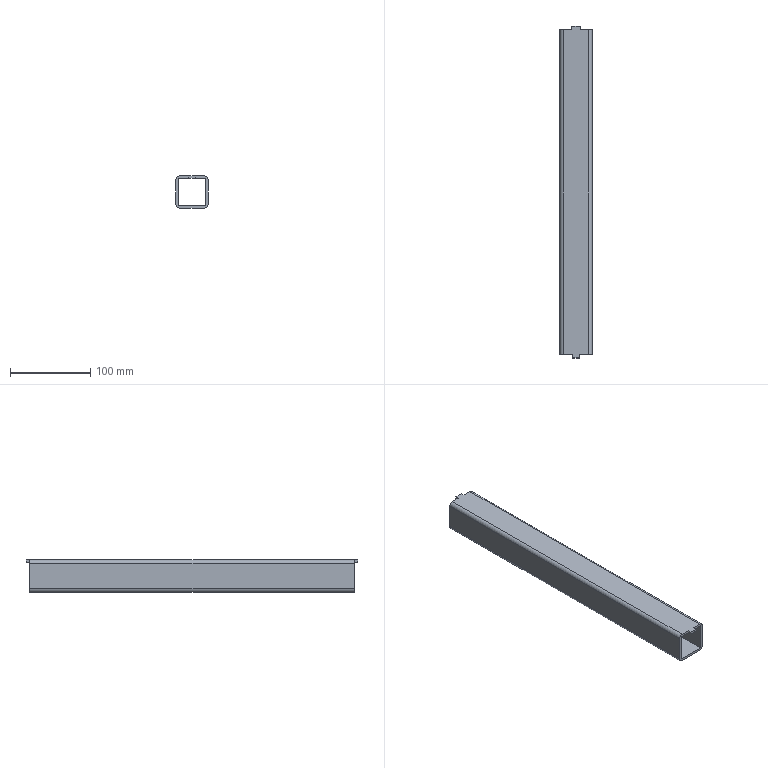Part | 1 solid | 20 faces | box 40 x 414 x 40 mm | volume 173023 mm3 | plane 16 | cylinder 4 | commonest cylinder face diameters 9 x4
STEP:
#1=CARTESIAN_POINT('',(-268.,85.,604.5));
#2=VERTEX_POINT('',#1);
#3=CARTESIAN_POINT('',(-268.,85.,635.5));
#4=VERTEX_POINT('',#3);
#5=CARTESIAN_POINT('',(-268.,85.,600.));
#6=DIRECTION('',(0.,0.,1.));
#7=VECTOR('',#6,1000.);
#8=LINE('',#5,#7);
#9=EDGE_CURVE('',#2,#4,#8,.T.);
#10=ORIENTED_EDGE('',*,*,#9,.F.);
#11=CARTESIAN_POINT('',(-268.,490.,604.5));
#12=VERTEX_POINT('',#11);
#13=CARTESIAN_POINT('',(-268.,490.,604.5));
#14=DIRECTION('',(0.,1.,0.));
#15=VECTOR('',#14,1000.);
#16=LINE('',#13,#15);
#17=EDGE_CURVE('',#2,#12,#16,.T.);
#18=ORIENTED_EDGE('',*,*,#17,.T.);
#19=CARTESIAN_POINT('',(-268.,490.,635.5));
#20=VERTEX_POINT('',#19);
#21=CARTESIAN_POINT('',(-268.,490.,600.));
#22=DIRECTION('',(0.,0.,1.));
#23=VECTOR('',#22,1000.);
#24=LINE('',#21,#23);
#25=EDGE_CURVE('',#12,#20,#24,.T.);
#26=ORIENTED_EDGE('',*,*,#25,.T.);
#27=CARTESIAN_POINT('',(-268.,40.,635.5));
#28=DIRECTION('',(0.,-1.,0.));
#29=VECTOR('',#28,1000.);
#30=LINE('',#27,#29);
#31=EDGE_CURVE('',#20,#4,#30,.T.);
#32=ORIENTED_EDGE('',*,*,#31,.T.);
#33=EDGE_LOOP('',(#10,#18,#26,#32));
#34=FACE_OUTER_BOUND('',#33,.T.);
#35=CARTESIAN_POINT('',(-268.,40.,600.));
#36=DIRECTION('',(1.,0.,0.));
#37=DIRECTION('',(0.,0.,-1.));
#38=AXIS2_PLACEMENT_3D('',#35,#36,#37);
#39=PLANE('',#38);
#40=ADVANCED_FACE('',(#34),#39,.T.);
#41=CARTESIAN_POINT('',(-308.,85.,604.5));
#42=VERTEX_POINT('',#41);
#43=CARTESIAN_POINT('',(-308.,85.,635.5));
#44=VERTEX_POINT('',#43);
#45=CARTESIAN_POINT('',(-308.,85.,600.));
#46=DIRECTION('',(0.,0.,1.));
#47=VECTOR('',#46,1000.);
#48=LINE('',#45,#47);
#49=EDGE_CURVE('',#42,#44,#48,.T.);
#50=ORIENTED_EDGE('',*,*,#49,.F.);
#51=CARTESIAN_POINT('',(-303.5,85.,600.));
#52=VERTEX_POINT('',#51);
#53=CARTESIAN_POINT('',(-303.5,85.,604.5));
#54=DIRECTION('',(0.,-1.,0.));
#55=DIRECTION('',(0.,0.,-1.));
#56=AXIS2_PLACEMENT_3D('',#53,#54,#55);
#57=CIRCLE('',#56,4.5);
#58=EDGE_CURVE('',#42,#52,#57,.T.);
#59=ORIENTED_EDGE('',*,*,#58,.T.);
#60=CARTESIAN_POINT('',(-272.5,85.,600.));
#61=VERTEX_POINT('',#60);
#62=CARTESIAN_POINT('',(-308.,85.,600.));
#63=DIRECTION('',(1.,0.,0.));
#64=VECTOR('',#63,1000.);
#65=LINE('',#62,#64);
#66=EDGE_CURVE('',#52,#61,#65,.T.);
#67=ORIENTED_EDGE('',*,*,#66,.T.);
#68=CARTESIAN_POINT('',(-272.5,85.,604.5));
#69=DIRECTION('',(0.,-1.,0.));
#70=DIRECTION('',(0.,0.,-1.));
#71=AXIS2_PLACEMENT_3D('',#68,#69,#70);
#72=CIRCLE('',#71,4.5);
#73=EDGE_CURVE('',#61,#2,#72,.T.);
#74=ORIENTED_EDGE('',*,*,#73,.T.);
#75=ORIENTED_EDGE('',*,*,#9,.T.);
#76=CARTESIAN_POINT('',(-272.5,85.,640.));
#77=VERTEX_POINT('',#76);
#78=CARTESIAN_POINT('',(-272.5,85.,635.5));
#79=DIRECTION('',(0.,-1.,0.));
#80=DIRECTION('',(0.,0.,-1.));
#81=AXIS2_PLACEMENT_3D('',#78,#79,#80);
#82=CIRCLE('',#81,4.5);
#83=EDGE_CURVE('',#4,#77,#82,.T.);
#84=ORIENTED_EDGE('',*,*,#83,.T.);
#85=CARTESIAN_POINT('',(-284.,85.,640.));
#86=VERTEX_POINT('',#85);
#87=CARTESIAN_POINT('',(-308.,85.,640.));
#88=DIRECTION('',(1.,0.,0.));
#89=VECTOR('',#88,1000.);
#90=LINE('',#87,#89);
#91=EDGE_CURVE('',#86,#77,#90,.T.);
#92=ORIENTED_EDGE('',*,*,#91,.F.);
#93=CARTESIAN_POINT('',(-284.,85.,637.));
#94=VERTEX_POINT('',#93);
#95=CARTESIAN_POINT('',(-284.,85.,640.));
#96=DIRECTION('',(0.,0.,1.));
#97=VECTOR('',#96,1000.);
#98=LINE('',#95,#97);
#99=EDGE_CURVE('',#94,#86,#98,.T.);
#100=ORIENTED_EDGE('',*,*,#99,.F.);
#101=CARTESIAN_POINT('',(-271.,85.,637.));
#102=VERTEX_POINT('',#101);
#103=CARTESIAN_POINT('',(-305.,85.,637.));
#104=DIRECTION('',(1.,0.,0.));
#105=VECTOR('',#104,1000.);
#106=LINE('',#103,#105);
#107=EDGE_CURVE('',#94,#102,#106,.T.);
#108=ORIENTED_EDGE('',*,*,#107,.T.);
#109=CARTESIAN_POINT('',(-271.,85.,603.));
#110=VERTEX_POINT('',#109);
#111=CARTESIAN_POINT('',(-271.,85.,637.));
#112=DIRECTION('',(0.,0.,-1.));
#113=VECTOR('',#112,1000.);
#114=LINE('',#111,#113);
#115=EDGE_CURVE('',#102,#110,#114,.T.);
#116=ORIENTED_EDGE('',*,*,#115,.T.);
#117=CARTESIAN_POINT('',(-305.,85.,603.));
#118=VERTEX_POINT('',#117);
#119=CARTESIAN_POINT('',(-271.,85.,603.));
#120=DIRECTION('',(-1.,0.,0.));
#121=VECTOR('',#120,1000.);
#122=LINE('',#119,#121);
#123=EDGE_CURVE('',#110,#118,#122,.T.);
#124=ORIENTED_EDGE('',*,*,#123,.T.);
#125=CARTESIAN_POINT('',(-305.,85.,637.));
#126=VERTEX_POINT('',#125);
#127=CARTESIAN_POINT('',(-305.,85.,603.));
#128=DIRECTION('',(0.,0.,1.));
#129=VECTOR('',#128,1000.);
#130=LINE('',#127,#129);
#131=EDGE_CURVE('',#118,#126,#130,.T.);
#132=ORIENTED_EDGE('',*,*,#131,.T.);
#133=CARTESIAN_POINT('',(-292.,85.,637.));
#134=VERTEX_POINT('',#133);
#135=CARTESIAN_POINT('',(-305.,85.,637.));
#136=DIRECTION('',(1.,0.,0.));
#137=VECTOR('',#136,1000.);
#138=LINE('',#135,#137);
#139=EDGE_CURVE('',#126,#134,#138,.T.);
#140=ORIENTED_EDGE('',*,*,#139,.T.);
#141=CARTESIAN_POINT('',(-292.,85.,640.));
#142=VERTEX_POINT('',#141);
#143=CARTESIAN_POINT('',(-292.,85.,637.));
#144=DIRECTION('',(0.,0.,-1.));
#145=VECTOR('',#144,1000.);
#146=LINE('',#143,#145);
#147=EDGE_CURVE('',#142,#134,#146,.T.);
#148=ORIENTED_EDGE('',*,*,#147,.F.);
#149=CARTESIAN_POINT('',(-303.5,85.,640.));
#150=VERTEX_POINT('',#149);
#151=CARTESIAN_POINT('',(-308.,85.,640.));
#152=DIRECTION('',(1.,0.,0.));
#153=VECTOR('',#152,1000.);
#154=LINE('',#151,#153);
#155=EDGE_CURVE('',#150,#142,#154,.T.);
#156=ORIENTED_EDGE('',*,*,#155,.F.);
#157=CARTESIAN_POINT('',(-303.5,85.,635.5));
#158=DIRECTION('',(0.,-1.,0.));
#159=DIRECTION('',(0.,0.,-1.));
#160=AXIS2_PLACEMENT_3D('',#157,#158,#159);
#161=CIRCLE('',#160,4.5);
#162=EDGE_CURVE('',#150,#44,#161,.T.);
#163=ORIENTED_EDGE('',*,*,#162,.T.);
#164=EDGE_LOOP('',(#50,#59,#67,#74,#75,#84,#92,#100,#108,#116,#124,#132,#140,#148,#156,#163));
#165=FACE_OUTER_BOUND('',#164,.T.);
#166=CARTESIAN_POINT('',(-308.,85.,600.));
#167=DIRECTION('',(0.,-1.,0.));
#168=DIRECTION('',(0.,0.,-1.));
#169=AXIS2_PLACEMENT_3D('',#166,#167,#168);
#170=PLANE('',#169);
#171=ADVANCED_FACE('',(#165),#170,.T.);
#172=CARTESIAN_POINT('',(-308.,490.,604.5));
#173=VERTEX_POINT('',#172);
#174=CARTESIAN_POINT('',(-308.,490.,635.5));
#175=VERTEX_POINT('',#174);
#176=CARTESIAN_POINT('',(-308.,490.,600.));
#177=DIRECTION('',(0.,0.,1.));
#178=VECTOR('',#177,1000.);
#179=LINE('',#176,#178);
#180=EDGE_CURVE('',#173,#175,#179,.T.);
#181=ORIENTED_EDGE('',*,*,#180,.F.);
#182=CARTESIAN_POINT('',(-308.,40.,604.5));
#183=DIRECTION('',(0.,-1.,0.));
#184=VECTOR('',#183,1000.);
#185=LINE('',#182,#184);
#186=EDGE_CURVE('',#173,#42,#185,.T.);
#187=ORIENTED_EDGE('',*,*,#186,.T.);
#188=ORIENTED_EDGE('',*,*,#49,.T.);
#189=CARTESIAN_POINT('',(-308.,490.,635.5));
#190=DIRECTION('',(0.,1.,0.));
#191=VECTOR('',#190,1000.);
#192=LINE('',#189,#191);
#193=EDGE_CURVE('',#44,#175,#192,.T.);
#194=ORIENTED_EDGE('',*,*,#193,.T.);
#195=EDGE_LOOP('',(#181,#187,#188,#194));
#196=FACE_OUTER_BOUND('',#195,.T.);
#197=CARTESIAN_POINT('',(-308.,490.,600.));
#198=DIRECTION('',(-1.,0.,0.));
#199=DIRECTION('',(0.,0.,1.));
#200=AXIS2_PLACEMENT_3D('',#197,#198,#199);
#201=PLANE('',#200);
#202=ADVANCED_FACE('',(#196),#201,.T.);
#203=CARTESIAN_POINT('',(-272.5,490.,600.));
#204=VERTEX_POINT('',#203);
#205=CARTESIAN_POINT('',(-303.5,490.,600.));
#206=VERTEX_POINT('',#205);
#207=CARTESIAN_POINT('',(-268.,490.,600.));
#208=DIRECTION('',(-1.,0.,0.));
#209=VECTOR('',#208,1000.);
#210=LINE('',#207,#209);
#211=EDGE_CURVE('',#204,#206,#210,.T.);
#212=ORIENTED_EDGE('',*,*,#211,.T.);
#213=CARTESIAN_POINT('',(-303.5,490.,604.5));
#214=DIRECTION('',(0.,1.,0.));
#215=DIRECTION('',(0.,0.,1.));
#216=AXIS2_PLACEMENT_3D('',#213,#214,#215);
#217=CIRCLE('',#216,4.5);
#218=EDGE_CURVE('',#206,#173,#217,.T.);
#219=ORIENTED_EDGE('',*,*,#218,.T.);
#220=ORIENTED_EDGE('',*,*,#180,.T.);
#221=CARTESIAN_POINT('',(-303.5,490.,640.));
#222=VERTEX_POINT('',#221);
#223=CARTESIAN_POINT('',(-303.5,490.,635.5));
#224=DIRECTION('',(0.,1.,0.));
#225=DIRECTION('',(0.,0.,1.));
#226=AXIS2_PLACEMENT_3D('',#223,#224,#225);
#227=CIRCLE('',#226,4.5);
#228=EDGE_CURVE('',#175,#222,#227,.T.);
#229=ORIENTED_EDGE('',*,*,#228,.T.);
#230=CARTESIAN_POINT('',(-293.,490.,640.));
#231=VERTEX_POINT('',#230);
#232=CARTESIAN_POINT('',(-268.,490.,640.));
#233=DIRECTION('',(-1.,0.,0.));
#234=VECTOR('',#233,1000.);
#235=LINE('',#232,#234);
#236=EDGE_CURVE('',#231,#222,#235,.T.);
#237=ORIENTED_EDGE('',*,*,#236,.F.);
#238=CARTESIAN_POINT('',(-293.,490.,637.));
#239=VERTEX_POINT('',#238);
#240=CARTESIAN_POINT('',(-293.,490.,640.));
#241=DIRECTION('',(0.,0.,1.));
#242=VECTOR('',#241,1000.);
#243=LINE('',#240,#242);
#244=EDGE_CURVE('',#239,#231,#243,.T.);
#245=ORIENTED_EDGE('',*,*,#244,.F.);
#246=CARTESIAN_POINT('',(-305.,490.,637.));
#247=VERTEX_POINT('',#246);
#248=CARTESIAN_POINT('',(-305.,490.,637.));
#249=DIRECTION('',(1.,0.,0.));
#250=VECTOR('',#249,1000.);
#251=LINE('',#248,#250);
#252=EDGE_CURVE('',#247,#239,#251,.T.);
#253=ORIENTED_EDGE('',*,*,#252,.F.);
#254=CARTESIAN_POINT('',(-305.,490.,603.));
#255=VERTEX_POINT('',#254);
#256=CARTESIAN_POINT('',(-305.,490.,603.));
#257=DIRECTION('',(0.,0.,1.));
#258=VECTOR('',#257,1000.);
#259=LINE('',#256,#258);
#260=EDGE_CURVE('',#255,#247,#259,.T.);
#261=ORIENTED_EDGE('',*,*,#260,.F.);
#262=CARTESIAN_POINT('',(-271.,490.,603.));
#263=VERTEX_POINT('',#262);
#264=CARTESIAN_POINT('',(-271.,490.,603.));
#265=DIRECTION('',(-1.,0.,0.));
#266=VECTOR('',#265,1000.);
#267=LINE('',#264,#266);
#268=EDGE_CURVE('',#263,#255,#267,.T.);
#269=ORIENTED_EDGE('',*,*,#268,.F.);
#270=CARTESIAN_POINT('',(-271.,490.,637.));
#271=VERTEX_POINT('',#270);
#272=CARTESIAN_POINT('',(-271.,490.,637.));
#273=DIRECTION('',(0.,0.,-1.));
#274=VECTOR('',#273,1000.);
#275=LINE('',#272,#274);
#276=EDGE_CURVE('',#271,#263,#275,.T.);
#277=ORIENTED_EDGE('',*,*,#276,.F.);
#278=CARTESIAN_POINT('',(-283.,490.,637.));
#279=VERTEX_POINT('',#278);
#280=CARTESIAN_POINT('',(-305.,490.,637.));
#281=DIRECTION('',(1.,0.,0.));
#282=VECTOR('',#281,1000.);
#283=LINE('',#280,#282);
#284=EDGE_CURVE('',#279,#271,#283,.T.);
#285=ORIENTED_EDGE('',*,*,#284,.F.);
#286=CARTESIAN_POINT('',(-283.,490.,640.));
#287=VERTEX_POINT('',#286);
#288=CARTESIAN_POINT('',(-283.,490.,637.));
#289=DIRECTION('',(0.,0.,-1.));
#290=VECTOR('',#289,1000.);
#291=LINE('',#288,#290);
#292=EDGE_CURVE('',#287,#279,#291,.T.);
#293=ORIENTED_EDGE('',*,*,#292,.F.);
#294=CARTESIAN_POINT('',(-272.5,490.,640.));
#295=VERTEX_POINT('',#294);
#296=CARTESIAN_POINT('',(-268.,490.,640.));
#297=DIRECTION('',(-1.,0.,0.));
#298=VECTOR('',#297,1000.);
#299=LINE('',#296,#298);
#300=EDGE_CURVE('',#295,#287,#299,.T.);
#301=ORIENTED_EDGE('',*,*,#300,.F.);
#302=CARTESIAN_POINT('',(-272.5,490.,635.5));
#303=DIRECTION('',(0.,1.,0.));
#304=DIRECTION('',(0.,0.,1.));
#305=AXIS2_PLACEMENT_3D('',#302,#303,#304);
#306=CIRCLE('',#305,4.5);
#307=EDGE_CURVE('',#295,#20,#306,.T.);
#308=ORIENTED_EDGE('',*,*,#307,.T.);
#309=ORIENTED_EDGE('',*,*,#25,.F.);
#310=CARTESIAN_POINT('',(-272.5,490.,604.5));
#311=DIRECTION('',(0.,1.,0.));
#312=DIRECTION('',(0.,0.,1.));
#313=AXIS2_PLACEMENT_3D('',#310,#311,#312);
#314=CIRCLE('',#313,4.5);
#315=EDGE_CURVE('',#12,#204,#314,.T.);
#316=ORIENTED_EDGE('',*,*,#315,.T.);
#317=EDGE_LOOP('',(#212,#219,#220,#229,#237,#245,#253,#261,#269,#277,#285,#293,#301,#308,#309,#316));
#318=FACE_OUTER_BOUND('',#317,.T.);
#319=CARTESIAN_POINT('',(-268.,490.,600.));
#320=DIRECTION('',(0.,1.,0.));
#321=DIRECTION('',(0.,0.,1.));
#322=AXIS2_PLACEMENT_3D('',#319,#320,#321);
#323=PLANE('',#322);
#324=ADVANCED_FACE('',(#318),#323,.T.);
#325=ORIENTED_EDGE('',*,*,#66,.F.);
#326=CARTESIAN_POINT('',(-303.5,490.,600.));
#327=DIRECTION('',(0.,1.,0.));
#328=VECTOR('',#327,1000.);
#329=LINE('',#326,#328);
#330=EDGE_CURVE('',#52,#206,#329,.T.);
#331=ORIENTED_EDGE('',*,*,#330,.T.);
#332=ORIENTED_EDGE('',*,*,#211,.F.);
#333=CARTESIAN_POINT('',(-272.5,40.,600.));
#334=DIRECTION('',(0.,-1.,0.));
#335=VECTOR('',#334,1000.);
#336=LINE('',#333,#335);
#337=EDGE_CURVE('',#204,#61,#336,.T.);
#338=ORIENTED_EDGE('',*,*,#337,.T.);
#339=EDGE_LOOP('',(#325,#331,#332,#338));
#340=FACE_OUTER_BOUND('',#339,.T.);
#341=CARTESIAN_POINT('',(0.,0.,600.));
#342=DIRECTION('',(0.,0.,1.));
#343=DIRECTION('',(1.,0.,0.));
#344=AXIS2_PLACEMENT_3D('',#341,#342,#343);
#345=PLANE('',#344);
#346=ADVANCED_FACE('',(#340),#345,.F.);
#347=ORIENTED_EDGE('',*,*,#236,.T.);
#348=CARTESIAN_POINT('',(-303.5,0.,640.));
#349=DIRECTION('',(0.,-1.,0.));
#350=VECTOR('',#349,1000.);
#351=LINE('',#348,#350);
#352=EDGE_CURVE('',#222,#150,#351,.T.);
#353=ORIENTED_EDGE('',*,*,#352,.T.);
#354=ORIENTED_EDGE('',*,*,#155,.T.);
#355=CARTESIAN_POINT('',(-292.,80.5,640.));
#356=VERTEX_POINT('',#355);
#357=CARTESIAN_POINT('',(-292.,80.5,640.));
#358=DIRECTION('',(0.,1.,0.));
#359=VECTOR('',#358,1000.);
#360=LINE('',#357,#359);
#361=EDGE_CURVE('',#356,#142,#360,.T.);
#362=ORIENTED_EDGE('',*,*,#361,.F.);
#363=CARTESIAN_POINT('',(-284.,80.5,640.));
#364=VERTEX_POINT('',#363);
#365=CARTESIAN_POINT('',(-292.,80.5,640.));
#366=DIRECTION('',(-1.,0.,0.));
#367=VECTOR('',#366,1000.);
#368=LINE('',#365,#367);
#369=EDGE_CURVE('',#364,#356,#368,.T.);
#370=ORIENTED_EDGE('',*,*,#369,.F.);
#371=CARTESIAN_POINT('',(-284.,80.5,640.));
#372=DIRECTION('',(0.,1.,0.));
#373=VECTOR('',#372,1000.);
#374=LINE('',#371,#373);
#375=EDGE_CURVE('',#364,#86,#374,.T.);
#376=ORIENTED_EDGE('',*,*,#375,.T.);
#377=ORIENTED_EDGE('',*,*,#91,.T.);
#378=CARTESIAN_POINT('',(-272.5,0.,640.));
#379=DIRECTION('',(0.,1.,0.));
#380=VECTOR('',#379,1000.);
#381=LINE('',#378,#380);
#382=EDGE_CURVE('',#77,#295,#381,.T.);
#383=ORIENTED_EDGE('',*,*,#382,.T.);
#384=ORIENTED_EDGE('',*,*,#300,.T.);
#385=CARTESIAN_POINT('',(-283.,494.5,640.));
#386=VERTEX_POINT('',#385);
#387=CARTESIAN_POINT('',(-283.,494.5,640.));
#388=DIRECTION('',(0.,-1.,0.));
#389=VECTOR('',#388,1000.);
#390=LINE('',#387,#389);
#391=EDGE_CURVE('',#386,#287,#390,.T.);
#392=ORIENTED_EDGE('',*,*,#391,.F.);
#393=CARTESIAN_POINT('',(-293.,494.5,640.));
#394=VERTEX_POINT('',#393);
#395=CARTESIAN_POINT('',(-283.,494.5,640.));
#396=DIRECTION('',(1.,0.,0.));
#397=VECTOR('',#396,1000.);
#398=LINE('',#395,#397);
#399=EDGE_CURVE('',#394,#386,#398,.T.);
#400=ORIENTED_EDGE('',*,*,#399,.F.);
#401=CARTESIAN_POINT('',(-293.,494.5,640.));
#402=DIRECTION('',(0.,-1.,0.));
#403=VECTOR('',#402,1000.);
#404=LINE('',#401,#403);
#405=EDGE_CURVE('',#394,#231,#404,.T.);
#406=ORIENTED_EDGE('',*,*,#405,.T.);
#407=EDGE_LOOP('',(#347,#353,#354,#362,#370,#376,#377,#383,#384,#392,#400,#406));
#408=FACE_OUTER_BOUND('',#407,.T.);
#409=CARTESIAN_POINT('',(0.,0.,640.));
#410=DIRECTION('',(0.,0.,1.));
#411=DIRECTION('',(1.,0.,0.));
#412=AXIS2_PLACEMENT_3D('',#409,#410,#411);
#413=PLANE('',#412);
#414=ADVANCED_FACE('',(#408),#413,.T.);
#415=ORIENTED_EDGE('',*,*,#252,.T.);
#416=CARTESIAN_POINT('',(-293.,494.5,637.));
#417=VERTEX_POINT('',#416);
#418=CARTESIAN_POINT('',(-293.,494.5,637.));
#419=DIRECTION('',(0.,-1.,0.));
#420=VECTOR('',#419,1000.);
#421=LINE('',#418,#420);
#422=EDGE_CURVE('',#417,#239,#421,.T.);
#423=ORIENTED_EDGE('',*,*,#422,.F.);
#424=CARTESIAN_POINT('',(-283.,494.5,637.));
#425=VERTEX_POINT('',#424);
#426=CARTESIAN_POINT('',(-293.,494.5,637.));
#427=DIRECTION('',(-1.,0.,0.));
#428=VECTOR('',#427,1000.);
#429=LINE('',#426,#428);
#430=EDGE_CURVE('',#425,#417,#429,.T.);
#431=ORIENTED_EDGE('',*,*,#430,.F.);
#432=CARTESIAN_POINT('',(-283.,494.5,637.));
#433=DIRECTION('',(0.,-1.,0.));
#434=VECTOR('',#433,1000.);
#435=LINE('',#432,#434);
#436=EDGE_CURVE('',#425,#279,#435,.T.);
#437=ORIENTED_EDGE('',*,*,#436,.T.);
#438=ORIENTED_EDGE('',*,*,#284,.T.);
#439=CARTESIAN_POINT('',(-271.,40.,637.));
#440=DIRECTION('',(0.,1.,0.));
#441=VECTOR('',#440,1000.);
#442=LINE('',#439,#441);
#443=EDGE_CURVE('',#102,#271,#442,.T.);
#444=ORIENTED_EDGE('',*,*,#443,.F.);
#445=ORIENTED_EDGE('',*,*,#107,.F.);
#446=CARTESIAN_POINT('',(-284.,80.5,637.));
#447=VERTEX_POINT('',#446);
#448=CARTESIAN_POINT('',(-284.,80.5,637.));
#449=DIRECTION('',(0.,1.,0.));
#450=VECTOR('',#449,1000.);
#451=LINE('',#448,#450);
#452=EDGE_CURVE('',#447,#94,#451,.T.);
#453=ORIENTED_EDGE('',*,*,#452,.F.);
#454=CARTESIAN_POINT('',(-292.,80.5,637.));
#455=VERTEX_POINT('',#454);
#456=CARTESIAN_POINT('',(-284.,80.5,637.));
#457=DIRECTION('',(1.,0.,0.));
#458=VECTOR('',#457,1000.);
#459=LINE('',#456,#458);
#460=EDGE_CURVE('',#455,#447,#459,.T.);
#461=ORIENTED_EDGE('',*,*,#460,.F.);
#462=CARTESIAN_POINT('',(-292.,80.5,637.));
#463=DIRECTION('',(0.,1.,0.));
#464=VECTOR('',#463,1000.);
#465=LINE('',#462,#464);
#466=EDGE_CURVE('',#455,#134,#465,.T.);
#467=ORIENTED_EDGE('',*,*,#466,.T.);
#468=ORIENTED_EDGE('',*,*,#139,.F.);
#469=CARTESIAN_POINT('',(-305.,40.,637.));
#470=DIRECTION('',(0.,1.,0.));
#471=VECTOR('',#470,1000.);
#472=LINE('',#469,#471);
#473=EDGE_CURVE('',#126,#247,#472,.T.);
#474=ORIENTED_EDGE('',*,*,#473,.T.);
#475=EDGE_LOOP('',(#415,#423,#431,#437,#438,#444,#445,#453,#461,#467,#468,#474));
#476=FACE_OUTER_BOUND('',#475,.T.);
#477=CARTESIAN_POINT('',(-305.,40.,637.));
#478=DIRECTION('',(0.,0.,1.));
#479=DIRECTION('',(1.,0.,0.));
#480=AXIS2_PLACEMENT_3D('',#477,#478,#479);
#481=PLANE('',#480);
#482=ADVANCED_FACE('',(#476),#481,.F.);
#483=ORIENTED_EDGE('',*,*,#260,.T.);
#484=ORIENTED_EDGE('',*,*,#473,.F.);
#485=ORIENTED_EDGE('',*,*,#131,.F.);
#486=CARTESIAN_POINT('',(-305.,40.,603.));
#487=DIRECTION('',(0.,1.,0.));
#488=VECTOR('',#487,1000.);
#489=LINE('',#486,#488);
#490=EDGE_CURVE('',#118,#255,#489,.T.);
#491=ORIENTED_EDGE('',*,*,#490,.T.);
#492=EDGE_LOOP('',(#483,#484,#485,#491));
#493=FACE_OUTER_BOUND('',#492,.T.);
#494=CARTESIAN_POINT('',(-305.,40.,603.));
#495=DIRECTION('',(-1.,0.,0.));
#496=DIRECTION('',(0.,0.,1.));
#497=AXIS2_PLACEMENT_3D('',#494,#495,#496);
#498=PLANE('',#497);
#499=ADVANCED_FACE('',(#493),#498,.F.);
#500=ORIENTED_EDGE('',*,*,#268,.T.);
#501=ORIENTED_EDGE('',*,*,#490,.F.);
#502=ORIENTED_EDGE('',*,*,#123,.F.);
#503=CARTESIAN_POINT('',(-271.,40.,603.));
#504=DIRECTION('',(0.,1.,0.));
#505=VECTOR('',#504,1000.);
#506=LINE('',#503,#505);
#507=EDGE_CURVE('',#110,#263,#506,.T.);
#508=ORIENTED_EDGE('',*,*,#507,.T.);
#509=EDGE_LOOP('',(#500,#501,#502,#508));
#510=FACE_OUTER_BOUND('',#509,.T.);
#511=CARTESIAN_POINT('',(-271.,40.,603.));
#512=DIRECTION('',(0.,0.,-1.));
#513=DIRECTION('',(-1.,0.,0.));
#514=AXIS2_PLACEMENT_3D('',#511,#512,#513);
#515=PLANE('',#514);
#516=ADVANCED_FACE('',(#510),#515,.F.);
#517=ORIENTED_EDGE('',*,*,#276,.T.);
#518=ORIENTED_EDGE('',*,*,#507,.F.);
#519=ORIENTED_EDGE('',*,*,#115,.F.);
#520=ORIENTED_EDGE('',*,*,#443,.T.);
#521=EDGE_LOOP('',(#517,#518,#519,#520));
#522=FACE_OUTER_BOUND('',#521,.T.);
#523=CARTESIAN_POINT('',(-271.,40.,637.));
#524=DIRECTION('',(1.,0.,0.));
#525=DIRECTION('',(0.,0.,-1.));
#526=AXIS2_PLACEMENT_3D('',#523,#524,#525);
#527=PLANE('',#526);
#528=ADVANCED_FACE('',(#522),#527,.F.);
#529=ORIENTED_EDGE('',*,*,#292,.T.);
#530=ORIENTED_EDGE('',*,*,#436,.F.);
#531=CARTESIAN_POINT('',(-283.,494.5,637.));
#532=DIRECTION('',(0.,0.,-1.));
#533=VECTOR('',#532,1000.);
#534=LINE('',#531,#533);
#535=EDGE_CURVE('',#386,#425,#534,.T.);
#536=ORIENTED_EDGE('',*,*,#535,.F.);
#537=ORIENTED_EDGE('',*,*,#391,.T.);
#538=EDGE_LOOP('',(#529,#530,#536,#537));
#539=FACE_OUTER_BOUND('',#538,.T.);
#540=CARTESIAN_POINT('',(-283.,494.5,637.));
#541=DIRECTION('',(-1.,0.,0.));
#542=DIRECTION('',(0.,0.,1.));
#543=AXIS2_PLACEMENT_3D('',#540,#541,#542);
#544=PLANE('',#543);
#545=ADVANCED_FACE('',(#539),#544,.F.);
#546=ORIENTED_EDGE('',*,*,#244,.T.);
#547=ORIENTED_EDGE('',*,*,#405,.F.);
#548=CARTESIAN_POINT('',(-293.,494.5,640.));
#549=DIRECTION('',(0.,0.,1.));
#550=VECTOR('',#549,1000.);
#551=LINE('',#548,#550);
#552=EDGE_CURVE('',#417,#394,#551,.T.);
#553=ORIENTED_EDGE('',*,*,#552,.F.);
#554=ORIENTED_EDGE('',*,*,#422,.T.);
#555=EDGE_LOOP('',(#546,#547,#553,#554));
#556=FACE_OUTER_BOUND('',#555,.T.);
#557=CARTESIAN_POINT('',(-293.,494.5,640.));
#558=DIRECTION('',(1.,0.,0.));
#559=DIRECTION('',(0.,0.,-1.));
#560=AXIS2_PLACEMENT_3D('',#557,#558,#559);
#561=PLANE('',#560);
#562=ADVANCED_FACE('',(#556),#561,.F.);
#563=ORIENTED_EDGE('',*,*,#535,.T.);
#564=ORIENTED_EDGE('',*,*,#430,.T.);
#565=ORIENTED_EDGE('',*,*,#552,.T.);
#566=ORIENTED_EDGE('',*,*,#399,.T.);
#567=EDGE_LOOP('',(#563,#564,#565,#566));
#568=FACE_OUTER_BOUND('',#567,.T.);
#569=CARTESIAN_POINT('',(0.,494.5,0.));
#570=DIRECTION('',(0.,-1.,0.));
#571=DIRECTION('',(0.,0.,-1.));
#572=AXIS2_PLACEMENT_3D('',#569,#570,#571);
#573=PLANE('',#572);
#574=ADVANCED_FACE('',(#568),#573,.F.);
#575=ORIENTED_EDGE('',*,*,#147,.T.);
#576=ORIENTED_EDGE('',*,*,#466,.F.);
#577=CARTESIAN_POINT('',(-292.,80.5,637.));
#578=DIRECTION('',(0.,0.,-1.));
#579=VECTOR('',#578,1000.);
#580=LINE('',#577,#579);
#581=EDGE_CURVE('',#356,#455,#580,.T.);
#582=ORIENTED_EDGE('',*,*,#581,.F.);
#583=ORIENTED_EDGE('',*,*,#361,.T.);
#584=EDGE_LOOP('',(#575,#576,#582,#583));
#585=FACE_OUTER_BOUND('',#584,.T.);
#586=CARTESIAN_POINT('',(-292.,80.5,637.));
#587=DIRECTION('',(1.,0.,0.));
#588=DIRECTION('',(0.,0.,-1.));
#589=AXIS2_PLACEMENT_3D('',#586,#587,#588);
#590=PLANE('',#589);
#591=ADVANCED_FACE('',(#585),#590,.F.);
#592=ORIENTED_EDGE('',*,*,#99,.T.);
#593=ORIENTED_EDGE('',*,*,#375,.F.);
#594=CARTESIAN_POINT('',(-284.,80.5,640.));
#595=DIRECTION('',(0.,0.,1.));
#596=VECTOR('',#595,1000.);
#597=LINE('',#594,#596);
#598=EDGE_CURVE('',#447,#364,#597,.T.);
#599=ORIENTED_EDGE('',*,*,#598,.F.);
#600=ORIENTED_EDGE('',*,*,#452,.T.);
#601=EDGE_LOOP('',(#592,#593,#599,#600));
#602=FACE_OUTER_BOUND('',#601,.T.);
#603=CARTESIAN_POINT('',(-284.,80.5,640.));
#604=DIRECTION('',(-1.,0.,0.));
#605=DIRECTION('',(0.,0.,1.));
#606=AXIS2_PLACEMENT_3D('',#603,#604,#605);
#607=PLANE('',#606);
#608=ADVANCED_FACE('',(#602),#607,.F.);
#609=ORIENTED_EDGE('',*,*,#581,.T.);
#610=ORIENTED_EDGE('',*,*,#460,.T.);
#611=ORIENTED_EDGE('',*,*,#598,.T.);
#612=ORIENTED_EDGE('',*,*,#369,.T.);
#613=EDGE_LOOP('',(#609,#610,#611,#612));
#614=FACE_OUTER_BOUND('',#613,.T.);
#615=CARTESIAN_POINT('',(0.,80.5,0.));
#616=DIRECTION('',(0.,1.,0.));
#617=DIRECTION('',(0.,0.,1.));
#618=AXIS2_PLACEMENT_3D('',#615,#616,#617);
#619=PLANE('',#618);
#620=ADVANCED_FACE('',(#614),#619,.F.);
#621=ORIENTED_EDGE('',*,*,#218,.F.);
#622=ORIENTED_EDGE('',*,*,#330,.F.);
#623=ORIENTED_EDGE('',*,*,#58,.F.);
#624=ORIENTED_EDGE('',*,*,#186,.F.);
#625=EDGE_LOOP('',(#621,#622,#623,#624));
#626=FACE_OUTER_BOUND('',#625,.T.);
#627=CARTESIAN_POINT('',(-303.5,490.,604.5));
#628=DIRECTION('',(0.,1.,0.));
#629=DIRECTION('',(0.,0.,1.));
#630=AXIS2_PLACEMENT_3D('',#627,#628,#629);
#631=CYLINDRICAL_SURFACE('',#630,4.5);
#632=ADVANCED_FACE('',(#626),#631,.T.);
#633=ORIENTED_EDGE('',*,*,#73,.F.);
#634=ORIENTED_EDGE('',*,*,#337,.F.);
#635=ORIENTED_EDGE('',*,*,#315,.F.);
#636=ORIENTED_EDGE('',*,*,#17,.F.);
#637=EDGE_LOOP('',(#633,#634,#635,#636));
#638=FACE_OUTER_BOUND('',#637,.T.);
#639=CARTESIAN_POINT('',(-272.5,40.,604.5));
#640=DIRECTION('',(0.,-1.,0.));
#641=DIRECTION('',(0.,0.,-1.));
#642=AXIS2_PLACEMENT_3D('',#639,#640,#641);
#643=CYLINDRICAL_SURFACE('',#642,4.5);
#644=ADVANCED_FACE('',(#638),#643,.T.);
#645=ORIENTED_EDGE('',*,*,#228,.F.);
#646=ORIENTED_EDGE('',*,*,#193,.F.);
#647=ORIENTED_EDGE('',*,*,#162,.F.);
#648=ORIENTED_EDGE('',*,*,#352,.F.);
#649=EDGE_LOOP('',(#645,#646,#647,#648));
#650=FACE_OUTER_BOUND('',#649,.T.);
#651=CARTESIAN_POINT('',(-303.5,0.,635.5));
#652=DIRECTION('',(0.,-1.,0.));
#653=DIRECTION('',(0.,0.,-1.));
#654=AXIS2_PLACEMENT_3D('',#651,#652,#653);
#655=CYLINDRICAL_SURFACE('',#654,4.5);
#656=ADVANCED_FACE('',(#650),#655,.T.);
#657=ORIENTED_EDGE('',*,*,#83,.F.);
#658=ORIENTED_EDGE('',*,*,#31,.F.);
#659=ORIENTED_EDGE('',*,*,#307,.F.);
#660=ORIENTED_EDGE('',*,*,#382,.F.);
#661=EDGE_LOOP('',(#657,#658,#659,#660));
#662=FACE_OUTER_BOUND('',#661,.T.);
#663=CARTESIAN_POINT('',(-272.5,0.,635.5));
#664=DIRECTION('',(0.,1.,0.));
#665=DIRECTION('',(0.,0.,1.));
#666=AXIS2_PLACEMENT_3D('',#663,#664,#665);
#667=CYLINDRICAL_SURFACE('',#666,4.5);
#668=ADVANCED_FACE('',(#662),#667,.T.);
#669=CLOSED_SHELL('',(#40,#171,#202,#324,#346,#414,#482,#499,#516,#528,#545,#562,#574,#591,#608,#620,#632,#644,#656,#668));
#670=MANIFOLD_SOLID_BREP('',#669);
#671=CARTESIAN_POINT('',(0.,0.,0.));
#672=DIRECTION('',(0.,0.,1.));
#673=DIRECTION('',(1.,0.,0.));
#674=AXIS2_PLACEMENT_3D('',#671,#672,#673);
#675=(LENGTH_UNIT()NAMED_UNIT(*)SI_UNIT(.MILLI.,.METRE.));
#676=UNCERTAINTY_MEASURE_WITH_UNIT(LENGTH_MEASURE(0.00001),#675,'','');
#677=(NAMED_UNIT(*)PLANE_ANGLE_UNIT()SI_UNIT($,.RADIAN.));
#678=(NAMED_UNIT(*)SI_UNIT($,.STERADIAN.)SOLID_ANGLE_UNIT());
#679=(GEOMETRIC_REPRESENTATION_CONTEXT(3)GLOBAL_UNCERTAINTY_ASSIGNED_CONTEXT((#676))GLOBAL_UNIT_ASSIGNED_CONTEXT((#675,#677,#678))REPRESENTATION_CONTEXT('',''));
#680=ADVANCED_BREP_SHAPE_REPRESENTATION('',(#670,#674),#679);